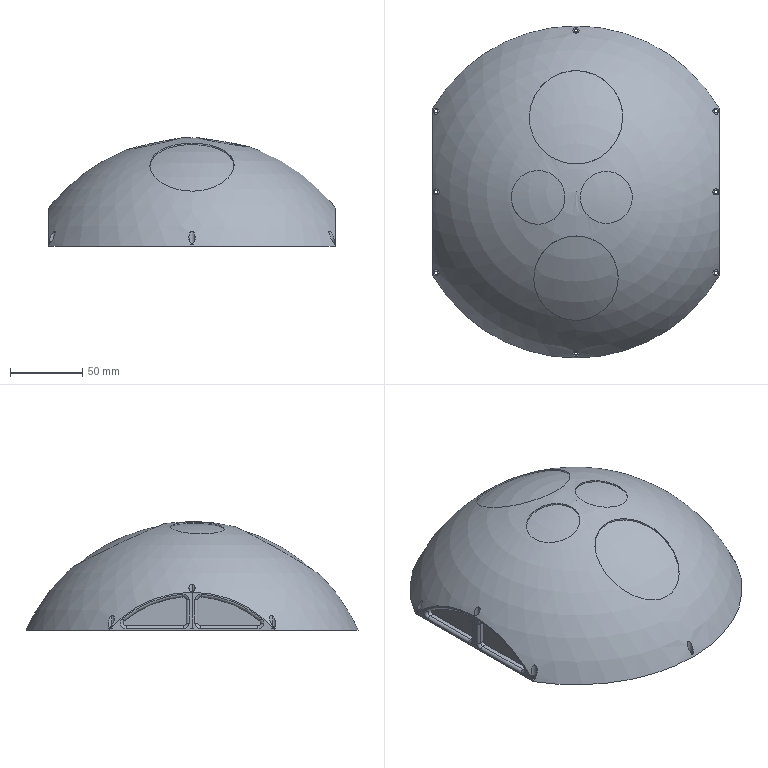Part | SolidWorks | features ICE 7, Fillet 2, Cut 1, MirrorPattern 1, OffsetRefSurface 1, Revolution 1, Shell 1 | 1 solid | 117 faces | box 198 x 229.129 x 75 mm | volume 126524 mm3 | cylinder 68 | plane 25 | torus 18 | sphere 6 | commonest cylinder face diameters 4 x22 2.3 x16 4.2 x16 146.63 x4 35.866 x2 37.039 x2